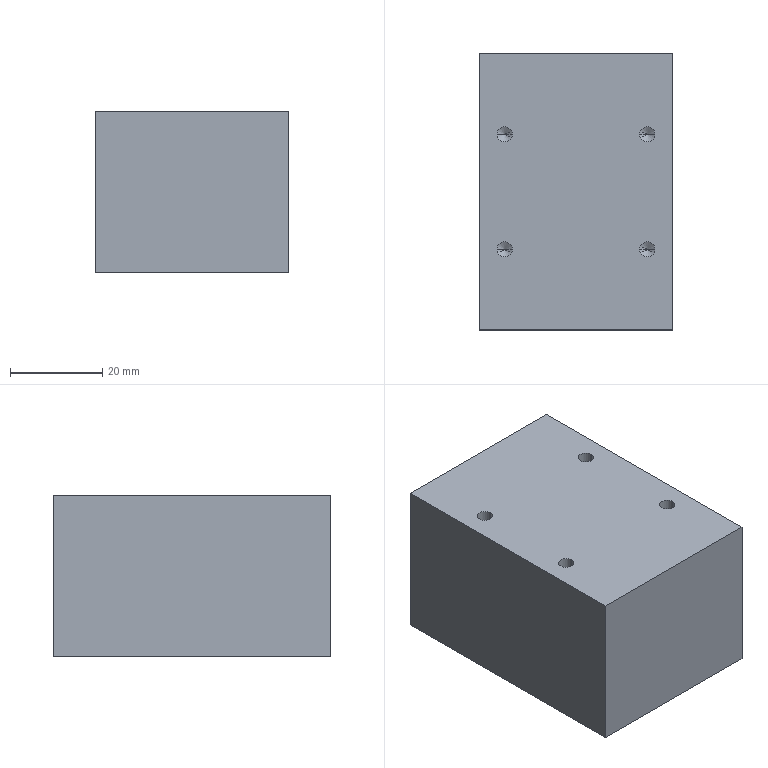Part | SolidWorks | features BaseBody 1 | 1 solid | 38 faces | box 42 x 60 x 35 mm | volume 86996 mm3 | cylinder 16 | cone 16 | plane 6 | commonest cylinder face diameters 3.3 x8 4.2 x8
STEP:
#1=CARTESIAN_POINT('',(-17.15,12.5,6.));
#2=VERTEX_POINT('',#1);
#3=CARTESIAN_POINT('',(-13.85,12.5,6.));
#4=VERTEX_POINT('',#3);
#5=CARTESIAN_POINT('',(-15.5,12.5,6.));
#6=DIRECTION('',(0.,0.,1.));
#7=DIRECTION('',(1.,0.,0.));
#8=AXIS2_PLACEMENT_3D('',#5,#6,#7);
#9=CIRCLE('',#8,1.65);
#10=EDGE_CURVE('',#2,#4,#9,.T.);
#11=ORIENTED_EDGE('',*,*,#10,.F.);
#12=CARTESIAN_POINT('',(-17.15,12.5,17.5));
#13=VERTEX_POINT('',#12);
#14=CARTESIAN_POINT('',(-17.15,12.5,17.5));
#15=DIRECTION('',(0.,0.,1.));
#16=VECTOR('',#15,1000.);
#17=LINE('',#14,#16);
#18=EDGE_CURVE('',#2,#13,#17,.T.);
#19=ORIENTED_EDGE('',*,*,#18,.T.);
#20=CARTESIAN_POINT('',(-13.85,12.5,17.5));
#21=VERTEX_POINT('',#20);
#22=CARTESIAN_POINT('',(-15.5,12.5,17.5));
#23=DIRECTION('',(0.,0.,1.));
#24=DIRECTION('',(1.,0.,0.));
#25=AXIS2_PLACEMENT_3D('',#22,#23,#24);
#26=CIRCLE('',#25,1.65);
#27=EDGE_CURVE('',#13,#21,#26,.T.);
#28=ORIENTED_EDGE('',*,*,#27,.T.);
#29=CARTESIAN_POINT('',(-13.85,12.5,17.5));
#30=DIRECTION('',(0.,0.,1.));
#31=VECTOR('',#30,1000.);
#32=LINE('',#29,#31);
#33=EDGE_CURVE('',#4,#21,#32,.T.);
#34=ORIENTED_EDGE('',*,*,#33,.F.);
#35=EDGE_LOOP('',(#11,#19,#28,#34));
#36=FACE_OUTER_BOUND('',#35,.T.);
#37=CARTESIAN_POINT('',(-15.5,12.5,17.5));
#38=DIRECTION('',(0.,0.,1.));
#39=DIRECTION('',(1.,0.,0.));
#40=AXIS2_PLACEMENT_3D('',#37,#38,#39);
#41=CYLINDRICAL_SURFACE('',#40,1.65);
#42=ADVANCED_FACE('',(#36),#41,.F.);
#43=CARTESIAN_POINT('',(-15.5,12.5,5.009));
#44=VERTEX_POINT('',#43);
#45=CARTESIAN_POINT('',(-13.85,12.5,6.));
#46=DIRECTION('',(0.8572,0.,0.515));
#47=VECTOR('',#46,1000.);
#48=LINE('',#45,#47);
#49=EDGE_CURVE('',#44,#4,#48,.T.);
#50=ORIENTED_EDGE('',*,*,#49,.F.);
#51=CARTESIAN_POINT('',(-17.15,12.5,6.));
#52=DIRECTION('',(-0.8572,0.,0.515));
#53=VECTOR('',#52,1000.);
#54=LINE('',#51,#53);
#55=EDGE_CURVE('',#44,#2,#54,.T.);
#56=ORIENTED_EDGE('',*,*,#55,.T.);
#57=ORIENTED_EDGE('',*,*,#10,.T.);
#58=EDGE_LOOP('',(#50,#56,#57));
#59=FACE_OUTER_BOUND('',#58,.T.);
#60=CARTESIAN_POINT('',(-15.5,12.5,6.));
#61=DIRECTION('',(0.,0.,1.));
#62=DIRECTION('',(1.,0.,0.));
#63=AXIS2_PLACEMENT_3D('',#60,#61,#62);
#64=CONICAL_SURFACE('',#63,1.65,1.03);
#65=ADVANCED_FACE('',(#59),#64,.F.);
#66=CARTESIAN_POINT('',(13.85,12.5,6.));
#67=VERTEX_POINT('',#66);
#68=CARTESIAN_POINT('',(17.15,12.5,6.));
#69=VERTEX_POINT('',#68);
#70=CARTESIAN_POINT('',(15.5,12.5,6.));
#71=DIRECTION('',(0.,0.,1.));
#72=DIRECTION('',(1.,0.,0.));
#73=AXIS2_PLACEMENT_3D('',#70,#71,#72);
#74=CIRCLE('',#73,1.65);
#75=EDGE_CURVE('',#67,#69,#74,.T.);
#76=ORIENTED_EDGE('',*,*,#75,.F.);
#77=CARTESIAN_POINT('',(13.85,12.5,17.5));
#78=VERTEX_POINT('',#77);
#79=CARTESIAN_POINT('',(13.85,12.5,17.5));
#80=DIRECTION('',(0.,0.,1.));
#81=VECTOR('',#80,1000.);
#82=LINE('',#79,#81);
#83=EDGE_CURVE('',#67,#78,#82,.T.);
#84=ORIENTED_EDGE('',*,*,#83,.T.);
#85=CARTESIAN_POINT('',(17.15,12.5,17.5));
#86=VERTEX_POINT('',#85);
#87=CARTESIAN_POINT('',(15.5,12.5,17.5));
#88=DIRECTION('',(0.,0.,1.));
#89=DIRECTION('',(1.,0.,0.));
#90=AXIS2_PLACEMENT_3D('',#87,#88,#89);
#91=CIRCLE('',#90,1.65);
#92=EDGE_CURVE('',#78,#86,#91,.T.);
#93=ORIENTED_EDGE('',*,*,#92,.T.);
#94=CARTESIAN_POINT('',(17.15,12.5,17.5));
#95=DIRECTION('',(0.,0.,1.));
#96=VECTOR('',#95,1000.);
#97=LINE('',#94,#96);
#98=EDGE_CURVE('',#69,#86,#97,.T.);
#99=ORIENTED_EDGE('',*,*,#98,.F.);
#100=EDGE_LOOP('',(#76,#84,#93,#99));
#101=FACE_OUTER_BOUND('',#100,.T.);
#102=CARTESIAN_POINT('',(15.5,12.5,17.5));
#103=DIRECTION('',(0.,0.,1.));
#104=DIRECTION('',(1.,0.,0.));
#105=AXIS2_PLACEMENT_3D('',#102,#103,#104);
#106=CYLINDRICAL_SURFACE('',#105,1.65);
#107=ADVANCED_FACE('',(#101),#106,.F.);
#108=CARTESIAN_POINT('',(15.5,12.5,5.009));
#109=VERTEX_POINT('',#108);
#110=CARTESIAN_POINT('',(17.15,12.5,6.));
#111=DIRECTION('',(0.8572,0.,0.515));
#112=VECTOR('',#111,1000.);
#113=LINE('',#110,#112);
#114=EDGE_CURVE('',#109,#69,#113,.T.);
#115=ORIENTED_EDGE('',*,*,#114,.F.);
#116=CARTESIAN_POINT('',(13.85,12.5,6.));
#117=DIRECTION('',(-0.8572,0.,0.515));
#118=VECTOR('',#117,1000.);
#119=LINE('',#116,#118);
#120=EDGE_CURVE('',#109,#67,#119,.T.);
#121=ORIENTED_EDGE('',*,*,#120,.T.);
#122=ORIENTED_EDGE('',*,*,#75,.T.);
#123=EDGE_LOOP('',(#115,#121,#122));
#124=FACE_OUTER_BOUND('',#123,.T.);
#125=CARTESIAN_POINT('',(15.5,12.5,6.));
#126=DIRECTION('',(0.,0.,1.));
#127=DIRECTION('',(1.,0.,0.));
#128=AXIS2_PLACEMENT_3D('',#125,#126,#127);
#129=CONICAL_SURFACE('',#128,1.65,1.03);
#130=ADVANCED_FACE('',(#124),#129,.F.);
#131=CARTESIAN_POINT('',(-17.15,-12.5,6.));
#132=VERTEX_POINT('',#131);
#133=CARTESIAN_POINT('',(-13.85,-12.5,6.));
#134=VERTEX_POINT('',#133);
#135=CARTESIAN_POINT('',(-15.5,-12.5,6.));
#136=DIRECTION('',(0.,0.,1.));
#137=DIRECTION('',(1.,0.,0.));
#138=AXIS2_PLACEMENT_3D('',#135,#136,#137);
#139=CIRCLE('',#138,1.65);
#140=EDGE_CURVE('',#132,#134,#139,.T.);
#141=ORIENTED_EDGE('',*,*,#140,.F.);
#142=CARTESIAN_POINT('',(-17.15,-12.5,17.5));
#143=VERTEX_POINT('',#142);
#144=CARTESIAN_POINT('',(-17.15,-12.5,17.5));
#145=DIRECTION('',(0.,0.,1.));
#146=VECTOR('',#145,1000.);
#147=LINE('',#144,#146);
#148=EDGE_CURVE('',#132,#143,#147,.T.);
#149=ORIENTED_EDGE('',*,*,#148,.T.);
#150=CARTESIAN_POINT('',(-13.85,-12.5,17.5));
#151=VERTEX_POINT('',#150);
#152=CARTESIAN_POINT('',(-15.5,-12.5,17.5));
#153=DIRECTION('',(0.,0.,1.));
#154=DIRECTION('',(1.,0.,0.));
#155=AXIS2_PLACEMENT_3D('',#152,#153,#154);
#156=CIRCLE('',#155,1.65);
#157=EDGE_CURVE('',#143,#151,#156,.T.);
#158=ORIENTED_EDGE('',*,*,#157,.T.);
#159=CARTESIAN_POINT('',(-13.85,-12.5,17.5));
#160=DIRECTION('',(0.,0.,1.));
#161=VECTOR('',#160,1000.);
#162=LINE('',#159,#161);
#163=EDGE_CURVE('',#134,#151,#162,.T.);
#164=ORIENTED_EDGE('',*,*,#163,.F.);
#165=EDGE_LOOP('',(#141,#149,#158,#164));
#166=FACE_OUTER_BOUND('',#165,.T.);
#167=CARTESIAN_POINT('',(-15.5,-12.5,17.5));
#168=DIRECTION('',(0.,0.,1.));
#169=DIRECTION('',(1.,0.,0.));
#170=AXIS2_PLACEMENT_3D('',#167,#168,#169);
#171=CYLINDRICAL_SURFACE('',#170,1.65);
#172=ADVANCED_FACE('',(#166),#171,.F.);
#173=CARTESIAN_POINT('',(-15.5,-12.5,5.009));
#174=VERTEX_POINT('',#173);
#175=CARTESIAN_POINT('',(-13.85,-12.5,6.));
#176=DIRECTION('',(0.8572,0.,0.515));
#177=VECTOR('',#176,1000.);
#178=LINE('',#175,#177);
#179=EDGE_CURVE('',#174,#134,#178,.T.);
#180=ORIENTED_EDGE('',*,*,#179,.F.);
#181=CARTESIAN_POINT('',(-17.15,-12.5,6.));
#182=DIRECTION('',(-0.8572,0.,0.515));
#183=VECTOR('',#182,1000.);
#184=LINE('',#181,#183);
#185=EDGE_CURVE('',#174,#132,#184,.T.);
#186=ORIENTED_EDGE('',*,*,#185,.T.);
#187=ORIENTED_EDGE('',*,*,#140,.T.);
#188=EDGE_LOOP('',(#180,#186,#187));
#189=FACE_OUTER_BOUND('',#188,.T.);
#190=CARTESIAN_POINT('',(-15.5,-12.5,6.));
#191=DIRECTION('',(0.,0.,1.));
#192=DIRECTION('',(1.,0.,0.));
#193=AXIS2_PLACEMENT_3D('',#190,#191,#192);
#194=CONICAL_SURFACE('',#193,1.65,1.03);
#195=ADVANCED_FACE('',(#189),#194,.F.);
#196=CARTESIAN_POINT('',(13.85,-12.5,6.));
#197=VERTEX_POINT('',#196);
#198=CARTESIAN_POINT('',(17.15,-12.5,6.));
#199=VERTEX_POINT('',#198);
#200=CARTESIAN_POINT('',(15.5,-12.5,6.));
#201=DIRECTION('',(0.,0.,1.));
#202=DIRECTION('',(1.,0.,0.));
#203=AXIS2_PLACEMENT_3D('',#200,#201,#202);
#204=CIRCLE('',#203,1.65);
#205=EDGE_CURVE('',#197,#199,#204,.T.);
#206=ORIENTED_EDGE('',*,*,#205,.F.);
#207=CARTESIAN_POINT('',(13.85,-12.5,17.5));
#208=VERTEX_POINT('',#207);
#209=CARTESIAN_POINT('',(13.85,-12.5,17.5));
#210=DIRECTION('',(0.,0.,1.));
#211=VECTOR('',#210,1000.);
#212=LINE('',#209,#211);
#213=EDGE_CURVE('',#197,#208,#212,.T.);
#214=ORIENTED_EDGE('',*,*,#213,.T.);
#215=CARTESIAN_POINT('',(17.15,-12.5,17.5));
#216=VERTEX_POINT('',#215);
#217=CARTESIAN_POINT('',(15.5,-12.5,17.5));
#218=DIRECTION('',(0.,0.,1.));
#219=DIRECTION('',(1.,0.,0.));
#220=AXIS2_PLACEMENT_3D('',#217,#218,#219);
#221=CIRCLE('',#220,1.65);
#222=EDGE_CURVE('',#208,#216,#221,.T.);
#223=ORIENTED_EDGE('',*,*,#222,.T.);
#224=CARTESIAN_POINT('',(17.15,-12.5,17.5));
#225=DIRECTION('',(0.,0.,1.));
#226=VECTOR('',#225,1000.);
#227=LINE('',#224,#226);
#228=EDGE_CURVE('',#199,#216,#227,.T.);
#229=ORIENTED_EDGE('',*,*,#228,.F.);
#230=EDGE_LOOP('',(#206,#214,#223,#229));
#231=FACE_OUTER_BOUND('',#230,.T.);
#232=CARTESIAN_POINT('',(15.5,-12.5,17.5));
#233=DIRECTION('',(0.,0.,1.));
#234=DIRECTION('',(1.,0.,0.));
#235=AXIS2_PLACEMENT_3D('',#232,#233,#234);
#236=CYLINDRICAL_SURFACE('',#235,1.65);
#237=ADVANCED_FACE('',(#231),#236,.F.);
#238=CARTESIAN_POINT('',(15.5,-12.5,5.009));
#239=VERTEX_POINT('',#238);
#240=CARTESIAN_POINT('',(17.15,-12.5,6.));
#241=DIRECTION('',(0.8572,0.,0.515));
#242=VECTOR('',#241,1000.);
#243=LINE('',#240,#242);
#244=EDGE_CURVE('',#239,#199,#243,.T.);
#245=ORIENTED_EDGE('',*,*,#244,.F.);
#246=CARTESIAN_POINT('',(13.85,-12.5,6.));
#247=DIRECTION('',(-0.8572,0.,0.515));
#248=VECTOR('',#247,1000.);
#249=LINE('',#246,#248);
#250=EDGE_CURVE('',#239,#197,#249,.T.);
#251=ORIENTED_EDGE('',*,*,#250,.T.);
#252=ORIENTED_EDGE('',*,*,#205,.T.);
#253=EDGE_LOOP('',(#245,#251,#252));
#254=FACE_OUTER_BOUND('',#253,.T.);
#255=CARTESIAN_POINT('',(15.5,-12.5,6.));
#256=DIRECTION('',(0.,0.,1.));
#257=DIRECTION('',(1.,0.,0.));
#258=AXIS2_PLACEMENT_3D('',#255,#256,#257);
#259=CONICAL_SURFACE('',#258,1.65,1.03);
#260=ADVANCED_FACE('',(#254),#259,.F.);
#261=CARTESIAN_POINT('',(17.1,-22.5,-3.5));
#262=VERTEX_POINT('',#261);
#263=CARTESIAN_POINT('',(12.9,-22.5,-3.5));
#264=VERTEX_POINT('',#263);
#265=CARTESIAN_POINT('',(15.,-22.5,-3.5));
#266=DIRECTION('',(0.,0.,-1.));
#267=DIRECTION('',(-1.,0.,0.));
#268=AXIS2_PLACEMENT_3D('',#265,#266,#267);
#269=CIRCLE('',#268,2.1);
#270=EDGE_CURVE('',#262,#264,#269,.T.);
#271=ORIENTED_EDGE('',*,*,#270,.F.);
#272=CARTESIAN_POINT('',(17.1,-22.5,-17.5));
#273=VERTEX_POINT('',#272);
#274=CARTESIAN_POINT('',(17.1,-22.5,-17.5));
#275=DIRECTION('',(0.,0.,-1.));
#276=VECTOR('',#275,1000.);
#277=LINE('',#274,#276);
#278=EDGE_CURVE('',#262,#273,#277,.T.);
#279=ORIENTED_EDGE('',*,*,#278,.T.);
#280=CARTESIAN_POINT('',(12.9,-22.5,-17.5));
#281=VERTEX_POINT('',#280);
#282=CARTESIAN_POINT('',(15.,-22.5,-17.5));
#283=DIRECTION('',(0.,0.,-1.));
#284=DIRECTION('',(-1.,0.,0.));
#285=AXIS2_PLACEMENT_3D('',#282,#283,#284);
#286=CIRCLE('',#285,2.1);
#287=EDGE_CURVE('',#273,#281,#286,.T.);
#288=ORIENTED_EDGE('',*,*,#287,.T.);
#289=CARTESIAN_POINT('',(12.9,-22.5,-17.5));
#290=DIRECTION('',(0.,0.,-1.));
#291=VECTOR('',#290,1000.);
#292=LINE('',#289,#291);
#293=EDGE_CURVE('',#264,#281,#292,.T.);
#294=ORIENTED_EDGE('',*,*,#293,.F.);
#295=EDGE_LOOP('',(#271,#279,#288,#294));
#296=FACE_OUTER_BOUND('',#295,.T.);
#297=CARTESIAN_POINT('',(15.,-22.5,-17.5));
#298=DIRECTION('',(0.,0.,-1.));
#299=DIRECTION('',(-1.,0.,0.));
#300=AXIS2_PLACEMENT_3D('',#297,#298,#299);
#301=CYLINDRICAL_SURFACE('',#300,2.1);
#302=ADVANCED_FACE('',(#296),#301,.F.);
#303=CARTESIAN_POINT('',(15.,-22.5,-2.238));
#304=VERTEX_POINT('',#303);
#305=CARTESIAN_POINT('',(12.9,-22.5,-3.5));
#306=DIRECTION('',(-0.8572,0.,-0.515));
#307=VECTOR('',#306,1000.);
#308=LINE('',#305,#307);
#309=EDGE_CURVE('',#304,#264,#308,.T.);
#310=ORIENTED_EDGE('',*,*,#309,.F.);
#311=CARTESIAN_POINT('',(17.1,-22.5,-3.5));
#312=DIRECTION('',(0.8572,0.,-0.515));
#313=VECTOR('',#312,1000.);
#314=LINE('',#311,#313);
#315=EDGE_CURVE('',#304,#262,#314,.T.);
#316=ORIENTED_EDGE('',*,*,#315,.T.);
#317=ORIENTED_EDGE('',*,*,#270,.T.);
#318=EDGE_LOOP('',(#310,#316,#317));
#319=FACE_OUTER_BOUND('',#318,.T.);
#320=CARTESIAN_POINT('',(15.,-22.5,-3.5));
#321=DIRECTION('',(0.,0.,-1.));
#322=DIRECTION('',(-1.,0.,0.));
#323=AXIS2_PLACEMENT_3D('',#320,#321,#322);
#324=CONICAL_SURFACE('',#323,2.1,1.03);
#325=ADVANCED_FACE('',(#319),#324,.F.);
#326=CARTESIAN_POINT('',(17.1,22.5,-3.5));
#327=VERTEX_POINT('',#326);
#328=CARTESIAN_POINT('',(12.9,22.5,-3.5));
#329=VERTEX_POINT('',#328);
#330=CARTESIAN_POINT('',(15.,22.5,-3.5));
#331=DIRECTION('',(0.,0.,-1.));
#332=DIRECTION('',(-1.,0.,0.));
#333=AXIS2_PLACEMENT_3D('',#330,#331,#332);
#334=CIRCLE('',#333,2.1);
#335=EDGE_CURVE('',#327,#329,#334,.T.);
#336=ORIENTED_EDGE('',*,*,#335,.F.);
#337=CARTESIAN_POINT('',(17.1,22.5,-17.5));
#338=VERTEX_POINT('',#337);
#339=CARTESIAN_POINT('',(17.1,22.5,-17.5));
#340=DIRECTION('',(0.,0.,-1.));
#341=VECTOR('',#340,1000.);
#342=LINE('',#339,#341);
#343=EDGE_CURVE('',#327,#338,#342,.T.);
#344=ORIENTED_EDGE('',*,*,#343,.T.);
#345=CARTESIAN_POINT('',(12.9,22.5,-17.5));
#346=VERTEX_POINT('',#345);
#347=CARTESIAN_POINT('',(15.,22.5,-17.5));
#348=DIRECTION('',(0.,0.,-1.));
#349=DIRECTION('',(-1.,0.,0.));
#350=AXIS2_PLACEMENT_3D('',#347,#348,#349);
#351=CIRCLE('',#350,2.1);
#352=EDGE_CURVE('',#338,#346,#351,.T.);
#353=ORIENTED_EDGE('',*,*,#352,.T.);
#354=CARTESIAN_POINT('',(12.9,22.5,-17.5));
#355=DIRECTION('',(0.,0.,-1.));
#356=VECTOR('',#355,1000.);
#357=LINE('',#354,#356);
#358=EDGE_CURVE('',#329,#346,#357,.T.);
#359=ORIENTED_EDGE('',*,*,#358,.F.);
#360=EDGE_LOOP('',(#336,#344,#353,#359));
#361=FACE_OUTER_BOUND('',#360,.T.);
#362=CARTESIAN_POINT('',(15.,22.5,-17.5));
#363=DIRECTION('',(0.,0.,-1.));
#364=DIRECTION('',(-1.,0.,0.));
#365=AXIS2_PLACEMENT_3D('',#362,#363,#364);
#366=CYLINDRICAL_SURFACE('',#365,2.1);
#367=ADVANCED_FACE('',(#361),#366,.F.);
#368=CARTESIAN_POINT('',(15.,22.5,-2.238));
#369=VERTEX_POINT('',#368);
#370=CARTESIAN_POINT('',(12.9,22.5,-3.5));
#371=DIRECTION('',(-0.8572,0.,-0.515));
#372=VECTOR('',#371,1000.);
#373=LINE('',#370,#372);
#374=EDGE_CURVE('',#369,#329,#373,.T.);
#375=ORIENTED_EDGE('',*,*,#374,.F.);
#376=CARTESIAN_POINT('',(17.1,22.5,-3.5));
#377=DIRECTION('',(0.8572,0.,-0.515));
#378=VECTOR('',#377,1000.);
#379=LINE('',#376,#378);
#380=EDGE_CURVE('',#369,#327,#379,.T.);
#381=ORIENTED_EDGE('',*,*,#380,.T.);
#382=ORIENTED_EDGE('',*,*,#335,.T.);
#383=EDGE_LOOP('',(#375,#381,#382));
#384=FACE_OUTER_BOUND('',#383,.T.);
#385=CARTESIAN_POINT('',(15.,22.5,-3.5));
#386=DIRECTION('',(0.,0.,-1.));
#387=DIRECTION('',(-1.,0.,0.));
#388=AXIS2_PLACEMENT_3D('',#385,#386,#387);
#389=CONICAL_SURFACE('',#388,2.1,1.03);
#390=ADVANCED_FACE('',(#384),#389,.F.);
#391=CARTESIAN_POINT('',(-12.9,-22.5,-3.5));
#392=VERTEX_POINT('',#391);
#393=CARTESIAN_POINT('',(-17.1,-22.5,-3.5));
#394=VERTEX_POINT('',#393);
#395=CARTESIAN_POINT('',(-15.,-22.5,-3.5));
#396=DIRECTION('',(0.,0.,-1.));
#397=DIRECTION('',(-1.,0.,0.));
#398=AXIS2_PLACEMENT_3D('',#395,#396,#397);
#399=CIRCLE('',#398,2.1);
#400=EDGE_CURVE('',#392,#394,#399,.T.);
#401=ORIENTED_EDGE('',*,*,#400,.F.);
#402=CARTESIAN_POINT('',(-12.9,-22.5,-17.5));
#403=VERTEX_POINT('',#402);
#404=CARTESIAN_POINT('',(-12.9,-22.5,-17.5));
#405=DIRECTION('',(0.,0.,-1.));
#406=VECTOR('',#405,1000.);
#407=LINE('',#404,#406);
#408=EDGE_CURVE('',#392,#403,#407,.T.);
#409=ORIENTED_EDGE('',*,*,#408,.T.);
#410=CARTESIAN_POINT('',(-17.1,-22.5,-17.5));
#411=VERTEX_POINT('',#410);
#412=CARTESIAN_POINT('',(-15.,-22.5,-17.5));
#413=DIRECTION('',(0.,0.,-1.));
#414=DIRECTION('',(-1.,0.,0.));
#415=AXIS2_PLACEMENT_3D('',#412,#413,#414);
#416=CIRCLE('',#415,2.1);
#417=EDGE_CURVE('',#403,#411,#416,.T.);
#418=ORIENTED_EDGE('',*,*,#417,.T.);
#419=CARTESIAN_POINT('',(-17.1,-22.5,-17.5));
#420=DIRECTION('',(0.,0.,-1.));
#421=VECTOR('',#420,1000.);
#422=LINE('',#419,#421);
#423=EDGE_CURVE('',#394,#411,#422,.T.);
#424=ORIENTED_EDGE('',*,*,#423,.F.);
#425=EDGE_LOOP('',(#401,#409,#418,#424));
#426=FACE_OUTER_BOUND('',#425,.T.);
#427=CARTESIAN_POINT('',(-15.,-22.5,-17.5));
#428=DIRECTION('',(0.,0.,-1.));
#429=DIRECTION('',(-1.,0.,0.));
#430=AXIS2_PLACEMENT_3D('',#427,#428,#429);
#431=CYLINDRICAL_SURFACE('',#430,2.1);
#432=ADVANCED_FACE('',(#426),#431,.F.);
#433=CARTESIAN_POINT('',(-15.,-22.5,-2.238));
#434=VERTEX_POINT('',#433);
#435=CARTESIAN_POINT('',(-17.1,-22.5,-3.5));
#436=DIRECTION('',(-0.8572,0.,-0.515));
#437=VECTOR('',#436,1000.);
#438=LINE('',#435,#437);
#439=EDGE_CURVE('',#434,#394,#438,.T.);
#440=ORIENTED_EDGE('',*,*,#439,.F.);
#441=CARTESIAN_POINT('',(-12.9,-22.5,-3.5));
#442=DIRECTION('',(0.8572,0.,-0.515));
#443=VECTOR('',#442,1000.);
#444=LINE('',#441,#443);
#445=EDGE_CURVE('',#434,#392,#444,.T.);
#446=ORIENTED_EDGE('',*,*,#445,.T.);
#447=ORIENTED_EDGE('',*,*,#400,.T.);
#448=EDGE_LOOP('',(#440,#446,#447));
#449=FACE_OUTER_BOUND('',#448,.T.);
#450=CARTESIAN_POINT('',(-15.,-22.5,-3.5));
#451=DIRECTION('',(0.,0.,-1.));
#452=DIRECTION('',(-1.,0.,0.));
#453=AXIS2_PLACEMENT_3D('',#450,#451,#452);
#454=CONICAL_SURFACE('',#453,2.1,1.03);
#455=ADVANCED_FACE('',(#449),#454,.F.);
#456=CARTESIAN_POINT('',(-12.9,22.5,-3.5));
#457=VERTEX_POINT('',#456);
#458=CARTESIAN_POINT('',(-17.1,22.5,-3.5));
#459=VERTEX_POINT('',#458);
#460=CARTESIAN_POINT('',(-15.,22.5,-3.5));
#461=DIRECTION('',(0.,0.,-1.));
#462=DIRECTION('',(-1.,0.,0.));
#463=AXIS2_PLACEMENT_3D('',#460,#461,#462);
#464=CIRCLE('',#463,2.1);
#465=EDGE_CURVE('',#457,#459,#464,.T.);
#466=ORIENTED_EDGE('',*,*,#465,.F.);
#467=CARTESIAN_POINT('',(-12.9,22.5,-17.5));
#468=VERTEX_POINT('',#467);
#469=CARTESIAN_POINT('',(-12.9,22.5,-17.5));
#470=DIRECTION('',(0.,0.,-1.));
#471=VECTOR('',#470,1000.);
#472=LINE('',#469,#471);
#473=EDGE_CURVE('',#457,#468,#472,.T.);
#474=ORIENTED_EDGE('',*,*,#473,.T.);
#475=CARTESIAN_POINT('',(-17.1,22.5,-17.5));
#476=VERTEX_POINT('',#475);
#477=CARTESIAN_POINT('',(-15.,22.5,-17.5));
#478=DIRECTION('',(0.,0.,-1.));
#479=DIRECTION('',(-1.,0.,0.));
#480=AXIS2_PLACEMENT_3D('',#477,#478,#479);
#481=CIRCLE('',#480,2.1);
#482=EDGE_CURVE('',#468,#476,#481,.T.);
#483=ORIENTED_EDGE('',*,*,#482,.T.);
#484=CARTESIAN_POINT('',(-17.1,22.5,-17.5));
#485=DIRECTION('',(0.,0.,-1.));
#486=VECTOR('',#485,1000.);
#487=LINE('',#484,#486);
#488=EDGE_CURVE('',#459,#476,#487,.T.);
#489=ORIENTED_EDGE('',*,*,#488,.F.);
#490=EDGE_LOOP('',(#466,#474,#483,#489));
#491=FACE_OUTER_BOUND('',#490,.T.);
#492=CARTESIAN_POINT('',(-15.,22.5,-17.5));
#493=DIRECTION('',(0.,0.,-1.));
#494=DIRECTION('',(-1.,0.,0.));
#495=AXIS2_PLACEMENT_3D('',#492,#493,#494);
#496=CYLINDRICAL_SURFACE('',#495,2.1);
#497=ADVANCED_FACE('',(#491),#496,.F.);
#498=CARTESIAN_POINT('',(-15.,22.5,-2.238));
#499=VERTEX_POINT('',#498);
#500=CARTESIAN_POINT('',(-17.1,22.5,-3.5));
#501=DIRECTION('',(-0.8572,0.,-0.515));
#502=VECTOR('',#501,1000.);
#503=LINE('',#500,#502);
#504=EDGE_CURVE('',#499,#459,#503,.T.);
#505=ORIENTED_EDGE('',*,*,#504,.F.);
#506=CARTESIAN_POINT('',(-12.9,22.5,-3.5));
#507=DIRECTION('',(0.8572,0.,-0.515));
#508=VECTOR('',#507,1000.);
#509=LINE('',#506,#508);
#510=EDGE_CURVE('',#499,#457,#509,.T.);
#511=ORIENTED_EDGE('',*,*,#510,.T.);
#512=ORIENTED_EDGE('',*,*,#465,.T.);
#513=EDGE_LOOP('',(#505,#511,#512));
#514=FACE_OUTER_BOUND('',#513,.T.);
#515=CARTESIAN_POINT('',(-15.,22.5,-3.5));
#516=DIRECTION('',(0.,0.,-1.));
#517=DIRECTION('',(-1.,0.,0.));
#518=AXIS2_PLACEMENT_3D('',#515,#516,#517);
#519=CONICAL_SURFACE('',#518,2.1,1.03);
#520=ADVANCED_FACE('',(#514),#519,.F.);
#521=CARTESIAN_POINT('',(-21.,30.,-17.5));
#522=VERTEX_POINT('',#521);
#523=CARTESIAN_POINT('',(-21.,-30.,-17.5));
#524=VERTEX_POINT('',#523);
#525=CARTESIAN_POINT('',(-21.,30.,-17.5));
#526=DIRECTION('',(0.,-1.,0.));
#527=VECTOR('',#526,1000.);
#528=LINE('',#525,#527);
#529=EDGE_CURVE('',#522,#524,#528,.T.);
#530=ORIENTED_EDGE('',*,*,#529,.T.);
#531=CARTESIAN_POINT('',(-21.,-30.,17.5));
#532=VERTEX_POINT('',#531);
#533=CARTESIAN_POINT('',(-21.,-30.,17.5));
#534=DIRECTION('',(0.,0.,-1.));
#535=VECTOR('',#534,1000.);
#536=LINE('',#533,#535);
#537=EDGE_CURVE('',#532,#524,#536,.T.);
#538=ORIENTED_EDGE('',*,*,#537,.F.);
#539=CARTESIAN_POINT('',(-21.,30.,17.5));
#540=VERTEX_POINT('',#539);
#541=CARTESIAN_POINT('',(-21.,30.,17.5));
#542=DIRECTION('',(0.,-1.,0.));
#543=VECTOR('',#542,1000.);
#544=LINE('',#541,#543);
#545=EDGE_CURVE('',#540,#532,#544,.T.);
#546=ORIENTED_EDGE('',*,*,#545,.F.);
#547=CARTESIAN_POINT('',(-21.,30.,17.5));
#548=DIRECTION('',(0.,0.,-1.));
#549=VECTOR('',#548,1000.);
#550=LINE('',#547,#549);
#551=EDGE_CURVE('',#540,#522,#550,.T.);
#552=ORIENTED_EDGE('',*,*,#551,.T.);
#553=EDGE_LOOP('',(#530,#538,#546,#552));
#554=FACE_OUTER_BOUND('',#553,.T.);
#555=CARTESIAN_POINT('',(-21.,30.,17.5));
#556=DIRECTION('',(1.,0.,0.));
#557=DIRECTION('',(0.,1.,0.));
#558=AXIS2_PLACEMENT_3D('',#555,#556,#557);
#559=PLANE('',#558);
#560=ADVANCED_FACE('',(#554),#559,.F.);
#561=CARTESIAN_POINT('',(21.,-30.,-17.5));
#562=VERTEX_POINT('',#561);
#563=CARTESIAN_POINT('',(21.,-30.,-17.5));
#564=DIRECTION('',(1.,0.,0.));
#565=VECTOR('',#564,1000.);
#566=LINE('',#563,#565);
#567=EDGE_CURVE('',#524,#562,#566,.T.);
#568=ORIENTED_EDGE('',*,*,#567,.T.);
#569=CARTESIAN_POINT('',(21.,-30.,17.5));
#570=VERTEX_POINT('',#569);
#571=CARTESIAN_POINT('',(21.,-30.,17.5));
#572=DIRECTION('',(0.,0.,-1.));
#573=VECTOR('',#572,1000.);
#574=LINE('',#571,#573);
#575=EDGE_CURVE('',#570,#562,#574,.T.);
#576=ORIENTED_EDGE('',*,*,#575,.F.);
#577=CARTESIAN_POINT('',(21.,-30.,17.5));
#578=DIRECTION('',(1.,0.,0.));
#579=VECTOR('',#578,1000.);
#580=LINE('',#577,#579);
#581=EDGE_CURVE('',#532,#570,#580,.T.);
#582=ORIENTED_EDGE('',*,*,#581,.F.);
#583=ORIENTED_EDGE('',*,*,#537,.T.);
#584=EDGE_LOOP('',(#568,#576,#582,#583));
#585=FACE_OUTER_BOUND('',#584,.T.);
#586=CARTESIAN_POINT('',(21.,-30.,17.5));
#587=DIRECTION('',(0.,1.,0.));
#588=DIRECTION('',(-1.,0.,0.));
#589=AXIS2_PLACEMENT_3D('',#586,#587,#588);
#590=PLANE('',#589);
#591=ADVANCED_FACE('',(#585),#590,.F.);
#592=CARTESIAN_POINT('',(21.,30.,-17.5));
#593=VERTEX_POINT('',#592);
#594=CARTESIAN_POINT('',(21.,30.,-17.5));
#595=DIRECTION('',(0.,1.,0.));
#596=VECTOR('',#595,1000.);
#597=LINE('',#594,#596);
#598=EDGE_CURVE('',#562,#593,#597,.T.);
#599=ORIENTED_EDGE('',*,*,#598,.T.);
#600=CARTESIAN_POINT('',(21.,30.,17.5));
#601=VERTEX_POINT('',#600);
#602=CARTESIAN_POINT('',(21.,30.,17.5));
#603=DIRECTION('',(0.,0.,-1.));
#604=VECTOR('',#603,1000.);
#605=LINE('',#602,#604);
#606=EDGE_CURVE('',#601,#593,#605,.T.);
#607=ORIENTED_EDGE('',*,*,#606,.F.);
#608=CARTESIAN_POINT('',(21.,30.,17.5));
#609=DIRECTION('',(0.,1.,0.));
#610=VECTOR('',#609,1000.);
#611=LINE('',#608,#610);
#612=EDGE_CURVE('',#570,#601,#611,.T.);
#613=ORIENTED_EDGE('',*,*,#612,.F.);
#614=ORIENTED_EDGE('',*,*,#575,.T.);
#615=EDGE_LOOP('',(#599,#607,#613,#614));
#616=FACE_OUTER_BOUND('',#615,.T.);
#617=CARTESIAN_POINT('',(21.,30.,17.5));
#618=DIRECTION('',(-1.,0.,0.));
#619=DIRECTION('',(0.,-1.,0.));
#620=AXIS2_PLACEMENT_3D('',#617,#618,#619);
#621=PLANE('',#620);
#622=ADVANCED_FACE('',(#616),#621,.F.);
#623=CARTESIAN_POINT('',(21.,30.,-17.5));
#624=DIRECTION('',(-1.,0.,0.));
#625=VECTOR('',#624,1000.);
#626=LINE('',#623,#625);
#627=EDGE_CURVE('',#593,#522,#626,.T.);
#628=ORIENTED_EDGE('',*,*,#627,.T.);
#629=ORIENTED_EDGE('',*,*,#551,.F.);
#630=CARTESIAN_POINT('',(21.,30.,17.5));
#631=DIRECTION('',(-1.,0.,0.));
#632=VECTOR('',#631,1000.);
#633=LINE('',#630,#632);
#634=EDGE_CURVE('',#601,#540,#633,.T.);
#635=ORIENTED_EDGE('',*,*,#634,.F.);
#636=ORIENTED_EDGE('',*,*,#606,.T.);
#637=EDGE_LOOP('',(#628,#629,#635,#636));
#638=FACE_OUTER_BOUND('',#637,.T.);
#639=CARTESIAN_POINT('',(21.,30.,17.5));
#640=DIRECTION('',(0.,-1.,0.));
#641=DIRECTION('',(1.,0.,0.));
#642=AXIS2_PLACEMENT_3D('',#639,#640,#641);
#643=PLANE('',#642);
#644=ADVANCED_FACE('',(#638),#643,.F.);
#645=CARTESIAN_POINT('',(-15.5,12.5,17.5));
#646=DIRECTION('',(0.,0.,1.));
#647=DIRECTION('',(1.,0.,0.));
#648=AXIS2_PLACEMENT_3D('',#645,#646,#647);
#649=CIRCLE('',#648,1.65);
#650=EDGE_CURVE('',#21,#13,#649,.T.);
#651=ORIENTED_EDGE('',*,*,#650,.F.);
#652=ORIENTED_EDGE('',*,*,#27,.F.);
#653=EDGE_LOOP('',(#651,#652));
#654=FACE_BOUND('',#653,.T.);
#655=CARTESIAN_POINT('',(15.5,12.5,17.5));
#656=DIRECTION('',(0.,0.,1.));
#657=DIRECTION('',(1.,0.,0.));
#658=AXIS2_PLACEMENT_3D('',#655,#656,#657);
#659=CIRCLE('',#658,1.65);
#660=EDGE_CURVE('',#86,#78,#659,.T.);
#661=ORIENTED_EDGE('',*,*,#660,.F.);
#662=ORIENTED_EDGE('',*,*,#92,.F.);
#663=EDGE_LOOP('',(#661,#662));
#664=FACE_BOUND('',#663,.T.);
#665=CARTESIAN_POINT('',(-15.5,-12.5,17.5));
#666=DIRECTION('',(0.,0.,1.));
#667=DIRECTION('',(1.,0.,0.));
#668=AXIS2_PLACEMENT_3D('',#665,#666,#667);
#669=CIRCLE('',#668,1.65);
#670=EDGE_CURVE('',#151,#143,#669,.T.);
#671=ORIENTED_EDGE('',*,*,#670,.F.);
#672=ORIENTED_EDGE('',*,*,#157,.F.);
#673=EDGE_LOOP('',(#671,#672));
#674=FACE_BOUND('',#673,.T.);
#675=CARTESIAN_POINT('',(15.5,-12.5,17.5));
#676=DIRECTION('',(0.,0.,1.));
#677=DIRECTION('',(1.,0.,0.));
#678=AXIS2_PLACEMENT_3D('',#675,#676,#677);
#679=CIRCLE('',#678,1.65);
#680=EDGE_CURVE('',#216,#208,#679,.T.);
#681=ORIENTED_EDGE('',*,*,#680,.F.);
#682=ORIENTED_EDGE('',*,*,#222,.F.);
#683=EDGE_LOOP('',(#681,#682));
#684=FACE_BOUND('',#683,.T.);
#685=ORIENTED_EDGE('',*,*,#545,.T.);
#686=ORIENTED_EDGE('',*,*,#581,.T.);
#687=ORIENTED_EDGE('',*,*,#612,.T.);
#688=ORIENTED_EDGE('',*,*,#634,.T.);
#689=EDGE_LOOP('',(#685,#686,#687,#688));
#690=FACE_OUTER_BOUND('',#689,.T.);
#691=CARTESIAN_POINT('',(-21.,-30.,17.5));
#692=DIRECTION('',(0.,0.,-1.));
#693=DIRECTION('',(-1.,0.,0.));
#694=AXIS2_PLACEMENT_3D('',#691,#692,#693);
#695=PLANE('',#694);
#696=ADVANCED_FACE('',(#654,#664,#674,#684,#690),#695,.F.);
#697=CARTESIAN_POINT('',(15.,-22.5,-17.5));
#698=DIRECTION('',(0.,0.,-1.));
#699=DIRECTION('',(-1.,0.,0.));
#700=AXIS2_PLACEMENT_3D('',#697,#698,#699);
#701=CIRCLE('',#700,2.1);
#702=EDGE_CURVE('',#281,#273,#701,.T.);
#703=ORIENTED_EDGE('',*,*,#702,.F.);
#704=ORIENTED_EDGE('',*,*,#287,.F.);
#705=EDGE_LOOP('',(#703,#704));
#706=FACE_BOUND('',#705,.T.);
#707=CARTESIAN_POINT('',(15.,22.5,-17.5));
#708=DIRECTION('',(0.,0.,-1.));
#709=DIRECTION('',(-1.,0.,0.));
#710=AXIS2_PLACEMENT_3D('',#707,#708,#709);
#711=CIRCLE('',#710,2.1);
#712=EDGE_CURVE('',#346,#338,#711,.T.);
#713=ORIENTED_EDGE('',*,*,#712,.F.);
#714=ORIENTED_EDGE('',*,*,#352,.F.);
#715=EDGE_LOOP('',(#713,#714));
#716=FACE_BOUND('',#715,.T.);
#717=CARTESIAN_POINT('',(-15.,-22.5,-17.5));
#718=DIRECTION('',(0.,0.,-1.));
#719=DIRECTION('',(-1.,0.,0.));
#720=AXIS2_PLACEMENT_3D('',#717,#718,#719);
#721=CIRCLE('',#720,2.1);
#722=EDGE_CURVE('',#411,#403,#721,.T.);
#723=ORIENTED_EDGE('',*,*,#722,.F.);
#724=ORIENTED_EDGE('',*,*,#417,.F.);
#725=EDGE_LOOP('',(#723,#724));
#726=FACE_BOUND('',#725,.T.);
#727=CARTESIAN_POINT('',(-15.,22.5,-17.5));
#728=DIRECTION('',(0.,0.,-1.));
#729=DIRECTION('',(-1.,0.,0.));
#730=AXIS2_PLACEMENT_3D('',#727,#728,#729);
#731=CIRCLE('',#730,2.1);
#732=EDGE_CURVE('',#476,#468,#731,.T.);
#733=ORIENTED_EDGE('',*,*,#732,.F.);
#734=ORIENTED_EDGE('',*,*,#482,.F.);
#735=EDGE_LOOP('',(#733,#734));
#736=FACE_BOUND('',#735,.T.);
#737=ORIENTED_EDGE('',*,*,#529,.F.);
#738=ORIENTED_EDGE('',*,*,#627,.F.);
#739=ORIENTED_EDGE('',*,*,#598,.F.);
#740=ORIENTED_EDGE('',*,*,#567,.F.);
#741=EDGE_LOOP('',(#737,#738,#739,#740));
#742=FACE_OUTER_BOUND('',#741,.T.);
#743=CARTESIAN_POINT('',(-21.,-30.,-17.5));
#744=DIRECTION('',(0.,0.,-1.));
#745=DIRECTION('',(-1.,0.,0.));
#746=AXIS2_PLACEMENT_3D('',#743,#744,#745);
#747=PLANE('',#746);
#748=ADVANCED_FACE('',(#706,#716,#726,#736,#742),#747,.T.);
#749=ORIENTED_EDGE('',*,*,#510,.F.);
#750=ORIENTED_EDGE('',*,*,#504,.T.);
#751=CARTESIAN_POINT('',(-15.,22.5,-3.5));
#752=DIRECTION('',(0.,0.,-1.));
#753=DIRECTION('',(-1.,0.,0.));
#754=AXIS2_PLACEMENT_3D('',#751,#752,#753);
#755=CIRCLE('',#754,2.1);
#756=EDGE_CURVE('',#459,#457,#755,.T.);
#757=ORIENTED_EDGE('',*,*,#756,.T.);
#758=EDGE_LOOP('',(#749,#750,#757));
#759=FACE_OUTER_BOUND('',#758,.T.);
#760=CARTESIAN_POINT('',(-15.,22.5,-3.5));
#761=DIRECTION('',(0.,0.,-1.));
#762=DIRECTION('',(-1.,0.,0.));
#763=AXIS2_PLACEMENT_3D('',#760,#761,#762);
#764=CONICAL_SURFACE('',#763,2.1,1.03);
#765=ADVANCED_FACE('',(#759),#764,.F.);
#766=ORIENTED_EDGE('',*,*,#473,.F.);
#767=ORIENTED_EDGE('',*,*,#756,.F.);
#768=ORIENTED_EDGE('',*,*,#488,.T.);
#769=ORIENTED_EDGE('',*,*,#732,.T.);
#770=EDGE_LOOP('',(#766,#767,#768,#769));
#771=FACE_OUTER_BOUND('',#770,.T.);
#772=CARTESIAN_POINT('',(-15.,22.5,-17.5));
#773=DIRECTION('',(0.,0.,-1.));
#774=DIRECTION('',(-1.,0.,0.));
#775=AXIS2_PLACEMENT_3D('',#772,#773,#774);
#776=CYLINDRICAL_SURFACE('',#775,2.1);
#777=ADVANCED_FACE('',(#771),#776,.F.);
#778=ORIENTED_EDGE('',*,*,#445,.F.);
#779=ORIENTED_EDGE('',*,*,#439,.T.);
#780=CARTESIAN_POINT('',(-15.,-22.5,-3.5));
#781=DIRECTION('',(0.,0.,-1.));
#782=DIRECTION('',(-1.,0.,0.));
#783=AXIS2_PLACEMENT_3D('',#780,#781,#782);
#784=CIRCLE('',#783,2.1);
#785=EDGE_CURVE('',#394,#392,#784,.T.);
#786=ORIENTED_EDGE('',*,*,#785,.T.);
#787=EDGE_LOOP('',(#778,#779,#786));
#788=FACE_OUTER_BOUND('',#787,.T.);
#789=CARTESIAN_POINT('',(-15.,-22.5,-3.5));
#790=DIRECTION('',(0.,0.,-1.));
#791=DIRECTION('',(-1.,0.,0.));
#792=AXIS2_PLACEMENT_3D('',#789,#790,#791);
#793=CONICAL_SURFACE('',#792,2.1,1.03);
#794=ADVANCED_FACE('',(#788),#793,.F.);
#795=ORIENTED_EDGE('',*,*,#408,.F.);
#796=ORIENTED_EDGE('',*,*,#785,.F.);
#797=ORIENTED_EDGE('',*,*,#423,.T.);
#798=ORIENTED_EDGE('',*,*,#722,.T.);
#799=EDGE_LOOP('',(#795,#796,#797,#798));
#800=FACE_OUTER_BOUND('',#799,.T.);
#801=CARTESIAN_POINT('',(-15.,-22.5,-17.5));
#802=DIRECTION('',(0.,0.,-1.));
#803=DIRECTION('',(-1.,0.,0.));
#804=AXIS2_PLACEMENT_3D('',#801,#802,#803);
#805=CYLINDRICAL_SURFACE('',#804,2.1);
#806=ADVANCED_FACE('',(#800),#805,.F.);
#807=ORIENTED_EDGE('',*,*,#380,.F.);
#808=ORIENTED_EDGE('',*,*,#374,.T.);
#809=CARTESIAN_POINT('',(15.,22.5,-3.5));
#810=DIRECTION('',(0.,0.,-1.));
#811=DIRECTION('',(-1.,0.,0.));
#812=AXIS2_PLACEMENT_3D('',#809,#810,#811);
#813=CIRCLE('',#812,2.1);
#814=EDGE_CURVE('',#329,#327,#813,.T.);
#815=ORIENTED_EDGE('',*,*,#814,.T.);
#816=EDGE_LOOP('',(#807,#808,#815));
#817=FACE_OUTER_BOUND('',#816,.T.);
#818=CARTESIAN_POINT('',(15.,22.5,-3.5));
#819=DIRECTION('',(0.,0.,-1.));
#820=DIRECTION('',(-1.,0.,0.));
#821=AXIS2_PLACEMENT_3D('',#818,#819,#820);
#822=CONICAL_SURFACE('',#821,2.1,1.03);
#823=ADVANCED_FACE('',(#817),#822,.F.);
#824=ORIENTED_EDGE('',*,*,#343,.F.);
#825=ORIENTED_EDGE('',*,*,#814,.F.);
#826=ORIENTED_EDGE('',*,*,#358,.T.);
#827=ORIENTED_EDGE('',*,*,#712,.T.);
#828=EDGE_LOOP('',(#824,#825,#826,#827));
#829=FACE_OUTER_BOUND('',#828,.T.);
#830=CARTESIAN_POINT('',(15.,22.5,-17.5));
#831=DIRECTION('',(0.,0.,-1.));
#832=DIRECTION('',(-1.,0.,0.));
#833=AXIS2_PLACEMENT_3D('',#830,#831,#832);
#834=CYLINDRICAL_SURFACE('',#833,2.1);
#835=ADVANCED_FACE('',(#829),#834,.F.);
#836=ORIENTED_EDGE('',*,*,#315,.F.);
#837=ORIENTED_EDGE('',*,*,#309,.T.);
#838=CARTESIAN_POINT('',(15.,-22.5,-3.5));
#839=DIRECTION('',(0.,0.,-1.));
#840=DIRECTION('',(-1.,0.,0.));
#841=AXIS2_PLACEMENT_3D('',#838,#839,#840);
#842=CIRCLE('',#841,2.1);
#843=EDGE_CURVE('',#264,#262,#842,.T.);
#844=ORIENTED_EDGE('',*,*,#843,.T.);
#845=EDGE_LOOP('',(#836,#837,#844));
#846=FACE_OUTER_BOUND('',#845,.T.);
#847=CARTESIAN_POINT('',(15.,-22.5,-3.5));
#848=DIRECTION('',(0.,0.,-1.));
#849=DIRECTION('',(-1.,0.,0.));
#850=AXIS2_PLACEMENT_3D('',#847,#848,#849);
#851=CONICAL_SURFACE('',#850,2.1,1.03);
#852=ADVANCED_FACE('',(#846),#851,.F.);
#853=ORIENTED_EDGE('',*,*,#278,.F.);
#854=ORIENTED_EDGE('',*,*,#843,.F.);
#855=ORIENTED_EDGE('',*,*,#293,.T.);
#856=ORIENTED_EDGE('',*,*,#702,.T.);
#857=EDGE_LOOP('',(#853,#854,#855,#856));
#858=FACE_OUTER_BOUND('',#857,.T.);
#859=CARTESIAN_POINT('',(15.,-22.5,-17.5));
#860=DIRECTION('',(0.,0.,-1.));
#861=DIRECTION('',(-1.,0.,0.));
#862=AXIS2_PLACEMENT_3D('',#859,#860,#861);
#863=CYLINDRICAL_SURFACE('',#862,2.1);
#864=ADVANCED_FACE('',(#858),#863,.F.);
#865=ORIENTED_EDGE('',*,*,#250,.F.);
#866=ORIENTED_EDGE('',*,*,#244,.T.);
#867=CARTESIAN_POINT('',(15.5,-12.5,6.));
#868=DIRECTION('',(0.,0.,1.));
#869=DIRECTION('',(1.,0.,0.));
#870=AXIS2_PLACEMENT_3D('',#867,#868,#869);
#871=CIRCLE('',#870,1.65);
#872=EDGE_CURVE('',#199,#197,#871,.T.);
#873=ORIENTED_EDGE('',*,*,#872,.T.);
#874=EDGE_LOOP('',(#865,#866,#873));
#875=FACE_OUTER_BOUND('',#874,.T.);
#876=CARTESIAN_POINT('',(15.5,-12.5,6.));
#877=DIRECTION('',(0.,0.,1.));
#878=DIRECTION('',(1.,0.,0.));
#879=AXIS2_PLACEMENT_3D('',#876,#877,#878);
#880=CONICAL_SURFACE('',#879,1.65,1.03);
#881=ADVANCED_FACE('',(#875),#880,.F.);
#882=ORIENTED_EDGE('',*,*,#213,.F.);
#883=ORIENTED_EDGE('',*,*,#872,.F.);
#884=ORIENTED_EDGE('',*,*,#228,.T.);
#885=ORIENTED_EDGE('',*,*,#680,.T.);
#886=EDGE_LOOP('',(#882,#883,#884,#885));
#887=FACE_OUTER_BOUND('',#886,.T.);
#888=CARTESIAN_POINT('',(15.5,-12.5,17.5));
#889=DIRECTION('',(0.,0.,1.));
#890=DIRECTION('',(1.,0.,0.));
#891=AXIS2_PLACEMENT_3D('',#888,#889,#890);
#892=CYLINDRICAL_SURFACE('',#891,1.65);
#893=ADVANCED_FACE('',(#887),#892,.F.);
#894=ORIENTED_EDGE('',*,*,#185,.F.);
#895=ORIENTED_EDGE('',*,*,#179,.T.);
#896=CARTESIAN_POINT('',(-15.5,-12.5,6.));
#897=DIRECTION('',(0.,0.,1.));
#898=DIRECTION('',(1.,0.,0.));
#899=AXIS2_PLACEMENT_3D('',#896,#897,#898);
#900=CIRCLE('',#899,1.65);
#901=EDGE_CURVE('',#134,#132,#900,.T.);
#902=ORIENTED_EDGE('',*,*,#901,.T.);
#903=EDGE_LOOP('',(#894,#895,#902));
#904=FACE_OUTER_BOUND('',#903,.T.);
#905=CARTESIAN_POINT('',(-15.5,-12.5,6.));
#906=DIRECTION('',(0.,0.,1.));
#907=DIRECTION('',(1.,0.,0.));
#908=AXIS2_PLACEMENT_3D('',#905,#906,#907);
#909=CONICAL_SURFACE('',#908,1.65,1.03);
#910=ADVANCED_FACE('',(#904),#909,.F.);
#911=ORIENTED_EDGE('',*,*,#148,.F.);
#912=ORIENTED_EDGE('',*,*,#901,.F.);
#913=ORIENTED_EDGE('',*,*,#163,.T.);
#914=ORIENTED_EDGE('',*,*,#670,.T.);
#915=EDGE_LOOP('',(#911,#912,#913,#914));
#916=FACE_OUTER_BOUND('',#915,.T.);
#917=CARTESIAN_POINT('',(-15.5,-12.5,17.5));
#918=DIRECTION('',(0.,0.,1.));
#919=DIRECTION('',(1.,0.,0.));
#920=AXIS2_PLACEMENT_3D('',#917,#918,#919);
#921=CYLINDRICAL_SURFACE('',#920,1.65);
#922=ADVANCED_FACE('',(#916),#921,.F.);
#923=ORIENTED_EDGE('',*,*,#120,.F.);
#924=ORIENTED_EDGE('',*,*,#114,.T.);
#925=CARTESIAN_POINT('',(15.5,12.5,6.));
#926=DIRECTION('',(0.,0.,1.));
#927=DIRECTION('',(1.,0.,0.));
#928=AXIS2_PLACEMENT_3D('',#925,#926,#927);
#929=CIRCLE('',#928,1.65);
#930=EDGE_CURVE('',#69,#67,#929,.T.);
#931=ORIENTED_EDGE('',*,*,#930,.T.);
#932=EDGE_LOOP('',(#923,#924,#931));
#933=FACE_OUTER_BOUND('',#932,.T.);
#934=CARTESIAN_POINT('',(15.5,12.5,6.));
#935=DIRECTION('',(0.,0.,1.));
#936=DIRECTION('',(1.,0.,0.));
#937=AXIS2_PLACEMENT_3D('',#934,#935,#936);
#938=CONICAL_SURFACE('',#937,1.65,1.03);
#939=ADVANCED_FACE('',(#933),#938,.F.);
#940=ORIENTED_EDGE('',*,*,#83,.F.);
#941=ORIENTED_EDGE('',*,*,#930,.F.);
#942=ORIENTED_EDGE('',*,*,#98,.T.);
#943=ORIENTED_EDGE('',*,*,#660,.T.);
#944=EDGE_LOOP('',(#940,#941,#942,#943));
#945=FACE_OUTER_BOUND('',#944,.T.);
#946=CARTESIAN_POINT('',(15.5,12.5,17.5));
#947=DIRECTION('',(0.,0.,1.));
#948=DIRECTION('',(1.,0.,0.));
#949=AXIS2_PLACEMENT_3D('',#946,#947,#948);
#950=CYLINDRICAL_SURFACE('',#949,1.65);
#951=ADVANCED_FACE('',(#945),#950,.F.);
#952=ORIENTED_EDGE('',*,*,#55,.F.);
#953=ORIENTED_EDGE('',*,*,#49,.T.);
#954=CARTESIAN_POINT('',(-15.5,12.5,6.));
#955=DIRECTION('',(0.,0.,1.));
#956=DIRECTION('',(1.,0.,0.));
#957=AXIS2_PLACEMENT_3D('',#954,#955,#956);
#958=CIRCLE('',#957,1.65);
#959=EDGE_CURVE('',#4,#2,#958,.T.);
#960=ORIENTED_EDGE('',*,*,#959,.T.);
#961=EDGE_LOOP('',(#952,#953,#960));
#962=FACE_OUTER_BOUND('',#961,.T.);
#963=CARTESIAN_POINT('',(-15.5,12.5,6.));
#964=DIRECTION('',(0.,0.,1.));
#965=DIRECTION('',(1.,0.,0.));
#966=AXIS2_PLACEMENT_3D('',#963,#964,#965);
#967=CONICAL_SURFACE('',#966,1.65,1.03);
#968=ADVANCED_FACE('',(#962),#967,.F.);
#969=ORIENTED_EDGE('',*,*,#18,.F.);
#970=ORIENTED_EDGE('',*,*,#959,.F.);
#971=ORIENTED_EDGE('',*,*,#33,.T.);
#972=ORIENTED_EDGE('',*,*,#650,.T.);
#973=EDGE_LOOP('',(#969,#970,#971,#972));
#974=FACE_OUTER_BOUND('',#973,.T.);
#975=CARTESIAN_POINT('',(-15.5,12.5,17.5));
#976=DIRECTION('',(0.,0.,1.));
#977=DIRECTION('',(1.,0.,0.));
#978=AXIS2_PLACEMENT_3D('',#975,#976,#977);
#979=CYLINDRICAL_SURFACE('',#978,1.65);
#980=ADVANCED_FACE('',(#974),#979,.F.);
#981=CLOSED_SHELL('',(#42,#65,#107,#130,#172,#195,#237,#260,#302,#325,#367,#390,#432,#455,#497,#520,#560,#591,#622,#644,#696,#748,#765,#777,#794,#806,#823,#835,#852,#864,#881,#893,#910,#922,#939,#951,#968,#980));
#982=MANIFOLD_SOLID_BREP('',#981);
#983=CARTESIAN_POINT('',(0.,0.,0.));
#984=DIRECTION('',(0.,0.,1.));
#985=DIRECTION('',(1.,0.,0.));
#986=AXIS2_PLACEMENT_3D('',#983,#984,#985);
#987=(LENGTH_UNIT()NAMED_UNIT(*)SI_UNIT(.MILLI.,.METRE.));
#988=UNCERTAINTY_MEASURE_WITH_UNIT(LENGTH_MEASURE(0.00001),#987,'','');
#989=(NAMED_UNIT(*)PLANE_ANGLE_UNIT()SI_UNIT($,.RADIAN.));
#990=(NAMED_UNIT(*)SI_UNIT($,.STERADIAN.)SOLID_ANGLE_UNIT());
#991=(GEOMETRIC_REPRESENTATION_CONTEXT(3)GLOBAL_UNCERTAINTY_ASSIGNED_CONTEXT((#988))GLOBAL_UNIT_ASSIGNED_CONTEXT((#987,#989,#990))REPRESENTATION_CONTEXT('',''));
#992=ADVANCED_BREP_SHAPE_REPRESENTATION('',(#982,#986),#991);